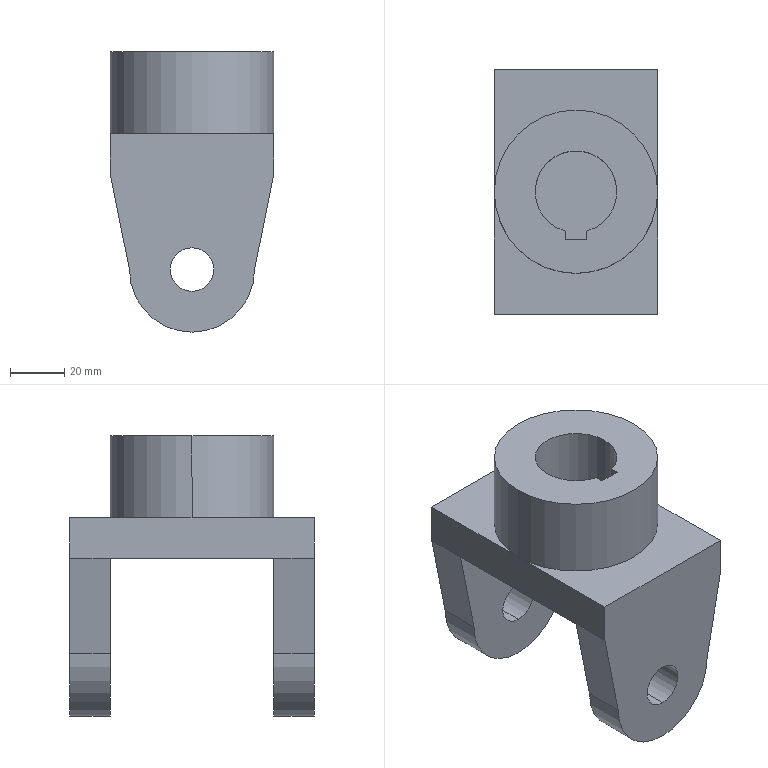Part | SolidWorks | features ICE 2, Extrusion 1, MirrorPattern 1 | 1 solid | 30 faces | box 60 x 90 x 103 mm | volume 218531 mm3 | plane 18 | cylinder 12 | commonest cylinder face diameters 16 x4 30 x3 46 x3 60 x2
STEP:
#1=CARTESIAN_POINT('',(4.,-14.457,30.));
#2=VERTEX_POINT('',#1);
#3=CARTESIAN_POINT('',(15.,0.,30.));
#4=VERTEX_POINT('',#3);
#5=CARTESIAN_POINT('',(0.,0.,30.));
#6=DIRECTION('',(0.,0.,1.));
#7=DIRECTION('',(1.,0.,0.));
#8=AXIS2_PLACEMENT_3D('',#5,#6,#7);
#9=CIRCLE('',#8,15.);
#10=EDGE_CURVE('',#2,#4,#9,.T.);
#11=ORIENTED_EDGE('',*,*,#10,.T.);
#12=CARTESIAN_POINT('',(15.,0.,0.));
#13=VERTEX_POINT('',#12);
#14=CARTESIAN_POINT('',(15.,0.,30.));
#15=DIRECTION('',(0.,0.,-1.));
#16=VECTOR('',#15,1000.);
#17=LINE('',#14,#16);
#18=EDGE_CURVE('',#4,#13,#17,.T.);
#19=ORIENTED_EDGE('',*,*,#18,.T.);
#20=CARTESIAN_POINT('',(4.,-14.457,0.));
#21=VERTEX_POINT('',#20);
#22=CARTESIAN_POINT('',(0.,0.,0.));
#23=DIRECTION('',(0.,0.,1.));
#24=DIRECTION('',(1.,0.,0.));
#25=AXIS2_PLACEMENT_3D('',#22,#23,#24);
#26=CIRCLE('',#25,15.);
#27=EDGE_CURVE('',#21,#13,#26,.T.);
#28=ORIENTED_EDGE('',*,*,#27,.F.);
#29=CARTESIAN_POINT('',(4.,-14.457,30.));
#30=DIRECTION('',(0.,0.,-1.));
#31=VECTOR('',#30,1000.);
#32=LINE('',#29,#31);
#33=EDGE_CURVE('',#2,#21,#32,.T.);
#34=ORIENTED_EDGE('',*,*,#33,.F.);
#35=EDGE_LOOP('',(#11,#19,#28,#34));
#36=FACE_OUTER_BOUND('',#35,.T.);
#37=CARTESIAN_POINT('',(0.,0.,30.));
#38=DIRECTION('',(0.,0.,-1.));
#39=DIRECTION('',(-1.,0.,0.));
#40=AXIS2_PLACEMENT_3D('',#37,#38,#39);
#41=CYLINDRICAL_SURFACE('',#40,15.);
#42=ADVANCED_FACE('',(#36),#41,.F.);
#43=ORIENTED_EDGE('',*,*,#18,.F.);
#44=CARTESIAN_POINT('',(-15.,0.,30.));
#45=VERTEX_POINT('',#44);
#46=CARTESIAN_POINT('',(0.,0.,30.));
#47=DIRECTION('',(0.,0.,1.));
#48=DIRECTION('',(1.,0.,0.));
#49=AXIS2_PLACEMENT_3D('',#46,#47,#48);
#50=CIRCLE('',#49,15.);
#51=EDGE_CURVE('',#4,#45,#50,.T.);
#52=ORIENTED_EDGE('',*,*,#51,.T.);
#53=CARTESIAN_POINT('',(-15.,0.,0.));
#54=VERTEX_POINT('',#53);
#55=CARTESIAN_POINT('',(-15.,0.,30.));
#56=DIRECTION('',(0.,0.,-1.));
#57=VECTOR('',#56,1000.);
#58=LINE('',#55,#57);
#59=EDGE_CURVE('',#45,#54,#58,.T.);
#60=ORIENTED_EDGE('',*,*,#59,.T.);
#61=CARTESIAN_POINT('',(0.,0.,0.));
#62=DIRECTION('',(0.,0.,1.));
#63=DIRECTION('',(1.,0.,0.));
#64=AXIS2_PLACEMENT_3D('',#61,#62,#63);
#65=CIRCLE('',#64,15.);
#66=EDGE_CURVE('',#13,#54,#65,.T.);
#67=ORIENTED_EDGE('',*,*,#66,.F.);
#68=EDGE_LOOP('',(#43,#52,#60,#67));
#69=FACE_OUTER_BOUND('',#68,.T.);
#70=CARTESIAN_POINT('',(0.,0.,30.));
#71=DIRECTION('',(0.,0.,-1.));
#72=DIRECTION('',(-1.,0.,0.));
#73=AXIS2_PLACEMENT_3D('',#70,#71,#72);
#74=CYLINDRICAL_SURFACE('',#73,15.);
#75=ADVANCED_FACE('',(#69),#74,.F.);
#76=CARTESIAN_POINT('',(30.,0.,30.));
#77=VERTEX_POINT('',#76);
#78=CARTESIAN_POINT('',(-30.,0.,30.));
#79=VERTEX_POINT('',#78);
#80=CARTESIAN_POINT('',(0.,0.,30.));
#81=DIRECTION('',(0.,0.,1.));
#82=DIRECTION('',(1.,0.,0.));
#83=AXIS2_PLACEMENT_3D('',#80,#81,#82);
#84=CIRCLE('',#83,30.);
#85=EDGE_CURVE('',#77,#79,#84,.T.);
#86=ORIENTED_EDGE('',*,*,#85,.F.);
#87=CARTESIAN_POINT('',(30.,0.,0.));
#88=VERTEX_POINT('',#87);
#89=CARTESIAN_POINT('',(30.,0.,30.));
#90=DIRECTION('',(0.,0.,-1.));
#91=VECTOR('',#90,1000.);
#92=LINE('',#89,#91);
#93=EDGE_CURVE('',#77,#88,#92,.T.);
#94=ORIENTED_EDGE('',*,*,#93,.T.);
#95=CARTESIAN_POINT('',(-30.,0.,0.));
#96=VERTEX_POINT('',#95);
#97=CARTESIAN_POINT('',(0.,0.,0.));
#98=DIRECTION('',(0.,0.,1.));
#99=DIRECTION('',(1.,0.,0.));
#100=AXIS2_PLACEMENT_3D('',#97,#98,#99);
#101=CIRCLE('',#100,30.);
#102=EDGE_CURVE('',#88,#96,#101,.T.);
#103=ORIENTED_EDGE('',*,*,#102,.T.);
#104=CARTESIAN_POINT('',(-30.,0.,30.));
#105=DIRECTION('',(0.,0.,-1.));
#106=VECTOR('',#105,1000.);
#107=LINE('',#104,#106);
#108=EDGE_CURVE('',#79,#96,#107,.T.);
#109=ORIENTED_EDGE('',*,*,#108,.F.);
#110=EDGE_LOOP('',(#86,#94,#103,#109));
#111=FACE_OUTER_BOUND('',#110,.T.);
#112=CARTESIAN_POINT('',(0.,0.,30.));
#113=DIRECTION('',(0.,0.,-1.));
#114=DIRECTION('',(-1.,0.,0.));
#115=AXIS2_PLACEMENT_3D('',#112,#113,#114);
#116=CYLINDRICAL_SURFACE('',#115,30.);
#117=ADVANCED_FACE('',(#111),#116,.T.);
#118=CARTESIAN_POINT('',(0.,-30.,-58.));
#119=VERTEX_POINT('',#118);
#120=CARTESIAN_POINT('',(0.,-30.,-42.));
#121=VERTEX_POINT('',#120);
#122=CARTESIAN_POINT('',(0.,-30.,-50.));
#123=DIRECTION('',(0.,1.,0.));
#124=DIRECTION('',(0.,0.,1.));
#125=AXIS2_PLACEMENT_3D('',#122,#123,#124);
#126=CIRCLE('',#125,8.);
#127=EDGE_CURVE('',#119,#121,#126,.T.);
#128=ORIENTED_EDGE('',*,*,#127,.T.);
#129=CARTESIAN_POINT('',(0.,-45.,-42.));
#130=VERTEX_POINT('',#129);
#131=CARTESIAN_POINT('',(0.,-30.,-42.));
#132=DIRECTION('',(0.,-1.,0.));
#133=VECTOR('',#132,1000.);
#134=LINE('',#131,#133);
#135=EDGE_CURVE('',#121,#130,#134,.T.);
#136=ORIENTED_EDGE('',*,*,#135,.T.);
#137=CARTESIAN_POINT('',(0.,-45.,-58.));
#138=VERTEX_POINT('',#137);
#139=CARTESIAN_POINT('',(0.,-45.,-50.));
#140=DIRECTION('',(0.,1.,0.));
#141=DIRECTION('',(0.,0.,1.));
#142=AXIS2_PLACEMENT_3D('',#139,#140,#141);
#143=CIRCLE('',#142,8.);
#144=EDGE_CURVE('',#138,#130,#143,.T.);
#145=ORIENTED_EDGE('',*,*,#144,.F.);
#146=CARTESIAN_POINT('',(0.,-30.,-58.));
#147=DIRECTION('',(0.,-1.,0.));
#148=VECTOR('',#147,1000.);
#149=LINE('',#146,#148);
#150=EDGE_CURVE('',#119,#138,#149,.T.);
#151=ORIENTED_EDGE('',*,*,#150,.F.);
#152=EDGE_LOOP('',(#128,#136,#145,#151));
#153=FACE_OUTER_BOUND('',#152,.T.);
#154=CARTESIAN_POINT('',(0.,-30.,-50.));
#155=DIRECTION('',(0.,-1.,0.));
#156=DIRECTION('',(0.,0.,-1.));
#157=AXIS2_PLACEMENT_3D('',#154,#155,#156);
#158=CYLINDRICAL_SURFACE('',#157,8.);
#159=ADVANCED_FACE('',(#153),#158,.F.);
#160=CARTESIAN_POINT('',(0.,-30.,-73.));
#161=VERTEX_POINT('',#160);
#162=CARTESIAN_POINT('',(-23.,-30.,-50.));
#163=VERTEX_POINT('',#162);
#164=CARTESIAN_POINT('',(0.,-30.,-50.));
#165=DIRECTION('',(0.,1.,0.));
#166=DIRECTION('',(0.,0.,1.));
#167=AXIS2_PLACEMENT_3D('',#164,#165,#166);
#168=CIRCLE('',#167,23.);
#169=EDGE_CURVE('',#161,#163,#168,.T.);
#170=ORIENTED_EDGE('',*,*,#169,.F.);
#171=CARTESIAN_POINT('',(0.,-45.,-73.));
#172=VERTEX_POINT('',#171);
#173=CARTESIAN_POINT('',(0.,-30.,-73.));
#174=DIRECTION('',(0.,-1.,0.));
#175=VECTOR('',#174,1000.);
#176=LINE('',#173,#175);
#177=EDGE_CURVE('',#161,#172,#176,.T.);
#178=ORIENTED_EDGE('',*,*,#177,.T.);
#179=CARTESIAN_POINT('',(-23.,-45.,-50.));
#180=VERTEX_POINT('',#179);
#181=CARTESIAN_POINT('',(0.,-45.,-50.));
#182=DIRECTION('',(0.,1.,0.));
#183=DIRECTION('',(0.,0.,1.));
#184=AXIS2_PLACEMENT_3D('',#181,#182,#183);
#185=CIRCLE('',#184,23.);
#186=EDGE_CURVE('',#172,#180,#185,.T.);
#187=ORIENTED_EDGE('',*,*,#186,.T.);
#188=CARTESIAN_POINT('',(-23.,-30.,-50.));
#189=DIRECTION('',(0.,-1.,0.));
#190=VECTOR('',#189,1000.);
#191=LINE('',#188,#190);
#192=EDGE_CURVE('',#163,#180,#191,.T.);
#193=ORIENTED_EDGE('',*,*,#192,.F.);
#194=EDGE_LOOP('',(#170,#178,#187,#193));
#195=FACE_OUTER_BOUND('',#194,.T.);
#196=CARTESIAN_POINT('',(0.,-30.,-50.));
#197=DIRECTION('',(0.,-1.,0.));
#198=DIRECTION('',(0.,0.,-1.));
#199=AXIS2_PLACEMENT_3D('',#196,#197,#198);
#200=CYLINDRICAL_SURFACE('',#199,23.);
#201=ADVANCED_FACE('',(#195),#200,.T.);
#202=CARTESIAN_POINT('',(0.,30.,-58.));
#203=VERTEX_POINT('',#202);
#204=CARTESIAN_POINT('',(0.,30.,-42.));
#205=VERTEX_POINT('',#204);
#206=CARTESIAN_POINT('',(0.,30.,-50.));
#207=DIRECTION('',(0.,1.,0.));
#208=DIRECTION('',(0.,0.,1.));
#209=AXIS2_PLACEMENT_3D('',#206,#207,#208);
#210=CIRCLE('',#209,8.);
#211=EDGE_CURVE('',#203,#205,#210,.T.);
#212=ORIENTED_EDGE('',*,*,#211,.F.);
#213=CARTESIAN_POINT('',(0.,45.,-58.));
#214=VERTEX_POINT('',#213);
#215=CARTESIAN_POINT('',(0.,30.,-58.));
#216=DIRECTION('',(0.,1.,0.));
#217=VECTOR('',#216,1000.);
#218=LINE('',#215,#217);
#219=EDGE_CURVE('',#203,#214,#218,.T.);
#220=ORIENTED_EDGE('',*,*,#219,.T.);
#221=CARTESIAN_POINT('',(0.,45.,-42.));
#222=VERTEX_POINT('',#221);
#223=CARTESIAN_POINT('',(0.,45.,-50.));
#224=DIRECTION('',(0.,1.,0.));
#225=DIRECTION('',(0.,0.,1.));
#226=AXIS2_PLACEMENT_3D('',#223,#224,#225);
#227=CIRCLE('',#226,8.);
#228=EDGE_CURVE('',#214,#222,#227,.T.);
#229=ORIENTED_EDGE('',*,*,#228,.T.);
#230=CARTESIAN_POINT('',(0.,30.,-42.));
#231=DIRECTION('',(0.,1.,0.));
#232=VECTOR('',#231,1000.);
#233=LINE('',#230,#232);
#234=EDGE_CURVE('',#205,#222,#233,.T.);
#235=ORIENTED_EDGE('',*,*,#234,.F.);
#236=EDGE_LOOP('',(#212,#220,#229,#235));
#237=FACE_OUTER_BOUND('',#236,.T.);
#238=CARTESIAN_POINT('',(0.,30.,-50.));
#239=DIRECTION('',(0.,1.,0.));
#240=DIRECTION('',(0.,0.,1.));
#241=AXIS2_PLACEMENT_3D('',#238,#239,#240);
#242=CYLINDRICAL_SURFACE('',#241,8.);
#243=ADVANCED_FACE('',(#237),#242,.F.);
#244=ORIENTED_EDGE('',*,*,#102,.F.);
#245=CARTESIAN_POINT('',(30.,45.,0.));
#246=VERTEX_POINT('',#245);
#247=CARTESIAN_POINT('',(30.,45.,0.));
#248=DIRECTION('',(0.,1.,0.));
#249=VECTOR('',#248,1000.);
#250=LINE('',#247,#249);
#251=EDGE_CURVE('',#88,#246,#250,.T.);
#252=ORIENTED_EDGE('',*,*,#251,.T.);
#253=CARTESIAN_POINT('',(-30.,45.,0.));
#254=VERTEX_POINT('',#253);
#255=CARTESIAN_POINT('',(-30.,45.,0.));
#256=DIRECTION('',(-1.,0.,0.));
#257=VECTOR('',#256,1000.);
#258=LINE('',#255,#257);
#259=EDGE_CURVE('',#246,#254,#258,.T.);
#260=ORIENTED_EDGE('',*,*,#259,.T.);
#261=CARTESIAN_POINT('',(-30.,45.,0.));
#262=DIRECTION('',(0.,-1.,0.));
#263=VECTOR('',#262,1000.);
#264=LINE('',#261,#263);
#265=EDGE_CURVE('',#254,#96,#264,.T.);
#266=ORIENTED_EDGE('',*,*,#265,.T.);
#267=EDGE_LOOP('',(#244,#252,#260,#266));
#268=FACE_OUTER_BOUND('',#267,.T.);
#269=CARTESIAN_POINT('',(0.,0.,0.));
#270=DIRECTION('',(0.,0.,1.));
#271=DIRECTION('',(1.,0.,0.));
#272=AXIS2_PLACEMENT_3D('',#269,#270,#271);
#273=PLANE('',#272);
#274=ADVANCED_FACE('',(#268),#273,.T.);
#275=CARTESIAN_POINT('',(-30.,-30.,-15.));
#276=VERTEX_POINT('',#275);
#277=CARTESIAN_POINT('',(30.,-30.,-15.));
#278=VERTEX_POINT('',#277);
#279=CARTESIAN_POINT('',(-30.,-30.,-15.));
#280=DIRECTION('',(1.,0.,0.));
#281=VECTOR('',#280,1000.);
#282=LINE('',#279,#281);
#283=EDGE_CURVE('',#276,#278,#282,.T.);
#284=ORIENTED_EDGE('',*,*,#283,.F.);
#285=CARTESIAN_POINT('',(-30.,30.,-15.));
#286=VERTEX_POINT('',#285);
#287=CARTESIAN_POINT('',(-30.,45.,-15.));
#288=DIRECTION('',(0.,-1.,0.));
#289=VECTOR('',#288,1000.);
#290=LINE('',#287,#289);
#291=EDGE_CURVE('',#286,#276,#290,.T.);
#292=ORIENTED_EDGE('',*,*,#291,.F.);
#293=CARTESIAN_POINT('',(30.,30.,-15.));
#294=VERTEX_POINT('',#293);
#295=CARTESIAN_POINT('',(-30.,30.,-15.));
#296=DIRECTION('',(1.,0.,0.));
#297=VECTOR('',#296,1000.);
#298=LINE('',#295,#297);
#299=EDGE_CURVE('',#286,#294,#298,.T.);
#300=ORIENTED_EDGE('',*,*,#299,.T.);
#301=CARTESIAN_POINT('',(30.,45.,-15.));
#302=DIRECTION('',(0.,1.,0.));
#303=VECTOR('',#302,1000.);
#304=LINE('',#301,#303);
#305=EDGE_CURVE('',#278,#294,#304,.T.);
#306=ORIENTED_EDGE('',*,*,#305,.F.);
#307=EDGE_LOOP('',(#284,#292,#300,#306));
#308=FACE_OUTER_BOUND('',#307,.T.);
#309=CARTESIAN_POINT('',(0.,0.,-15.));
#310=DIRECTION('',(0.,0.,1.));
#311=DIRECTION('',(1.,0.,0.));
#312=AXIS2_PLACEMENT_3D('',#309,#310,#311);
#313=PLANE('',#312);
#314=ADVANCED_FACE('',(#308),#313,.F.);
#315=CARTESIAN_POINT('',(30.,-45.,0.));
#316=VERTEX_POINT('',#315);
#317=CARTESIAN_POINT('',(30.,45.,0.));
#318=DIRECTION('',(0.,1.,0.));
#319=VECTOR('',#318,1000.);
#320=LINE('',#317,#319);
#321=EDGE_CURVE('',#316,#88,#320,.T.);
#322=ORIENTED_EDGE('',*,*,#321,.F.);
#323=CARTESIAN_POINT('',(30.,-45.,-15.));
#324=VERTEX_POINT('',#323);
#325=CARTESIAN_POINT('',(30.,-45.,-15.));
#326=DIRECTION('',(0.,0.,1.));
#327=VECTOR('',#326,1000.);
#328=LINE('',#325,#327);
#329=EDGE_CURVE('',#324,#316,#328,.T.);
#330=ORIENTED_EDGE('',*,*,#329,.F.);
#331=CARTESIAN_POINT('',(30.,45.,-15.));
#332=DIRECTION('',(0.,1.,0.));
#333=VECTOR('',#332,1000.);
#334=LINE('',#331,#333);
#335=EDGE_CURVE('',#324,#278,#334,.T.);
#336=ORIENTED_EDGE('',*,*,#335,.T.);
#337=ORIENTED_EDGE('',*,*,#305,.T.);
#338=CARTESIAN_POINT('',(30.,45.,-15.));
#339=VERTEX_POINT('',#338);
#340=CARTESIAN_POINT('',(30.,30.,-15.));
#341=DIRECTION('',(0.,1.,0.));
#342=VECTOR('',#341,1000.);
#343=LINE('',#340,#342);
#344=EDGE_CURVE('',#294,#339,#343,.T.);
#345=ORIENTED_EDGE('',*,*,#344,.T.);
#346=CARTESIAN_POINT('',(30.,45.,-15.));
#347=DIRECTION('',(0.,0.,1.));
#348=VECTOR('',#347,1000.);
#349=LINE('',#346,#348);
#350=EDGE_CURVE('',#339,#246,#349,.T.);
#351=ORIENTED_EDGE('',*,*,#350,.T.);
#352=ORIENTED_EDGE('',*,*,#251,.F.);
#353=EDGE_LOOP('',(#322,#330,#336,#337,#345,#351,#352));
#354=FACE_OUTER_BOUND('',#353,.T.);
#355=CARTESIAN_POINT('',(30.,45.,-15.));
#356=DIRECTION('',(1.,0.,0.));
#357=DIRECTION('',(0.,1.,0.));
#358=AXIS2_PLACEMENT_3D('',#355,#356,#357);
#359=PLANE('',#358);
#360=ADVANCED_FACE('',(#354),#359,.T.);
#361=CARTESIAN_POINT('',(-30.,-45.,0.));
#362=VERTEX_POINT('',#361);
#363=CARTESIAN_POINT('',(-30.,-45.,0.));
#364=DIRECTION('',(1.,0.,0.));
#365=VECTOR('',#364,1000.);
#366=LINE('',#363,#365);
#367=EDGE_CURVE('',#362,#316,#366,.T.);
#368=ORIENTED_EDGE('',*,*,#367,.F.);
#369=CARTESIAN_POINT('',(-30.,-45.,-15.));
#370=VERTEX_POINT('',#369);
#371=CARTESIAN_POINT('',(-30.,-45.,-15.));
#372=DIRECTION('',(0.,0.,1.));
#373=VECTOR('',#372,1000.);
#374=LINE('',#371,#373);
#375=EDGE_CURVE('',#370,#362,#374,.T.);
#376=ORIENTED_EDGE('',*,*,#375,.F.);
#377=CARTESIAN_POINT('',(-23.,-45.,-50.));
#378=DIRECTION('',(-0.1961,0.,0.9806));
#379=VECTOR('',#378,1000.);
#380=LINE('',#377,#379);
#381=EDGE_CURVE('',#180,#370,#380,.T.);
#382=ORIENTED_EDGE('',*,*,#381,.F.);
#383=ORIENTED_EDGE('',*,*,#186,.F.);
#384=CARTESIAN_POINT('',(23.,-45.,-50.));
#385=VERTEX_POINT('',#384);
#386=CARTESIAN_POINT('',(0.,-45.,-50.));
#387=DIRECTION('',(0.,1.,0.));
#388=DIRECTION('',(0.,0.,1.));
#389=AXIS2_PLACEMENT_3D('',#386,#387,#388);
#390=CIRCLE('',#389,23.);
#391=EDGE_CURVE('',#385,#172,#390,.T.);
#392=ORIENTED_EDGE('',*,*,#391,.F.);
#393=CARTESIAN_POINT('',(30.,-45.,-15.));
#394=DIRECTION('',(-0.1961,0.,-0.9806));
#395=VECTOR('',#394,1000.);
#396=LINE('',#393,#395);
#397=EDGE_CURVE('',#324,#385,#396,.T.);
#398=ORIENTED_EDGE('',*,*,#397,.F.);
#399=ORIENTED_EDGE('',*,*,#329,.T.);
#400=EDGE_LOOP('',(#368,#376,#382,#383,#392,#398,#399));
#401=FACE_OUTER_BOUND('',#400,.T.);
#402=ORIENTED_EDGE('',*,*,#144,.T.);
#403=CARTESIAN_POINT('',(0.,-45.,-50.));
#404=DIRECTION('',(0.,1.,0.));
#405=DIRECTION('',(0.,0.,1.));
#406=AXIS2_PLACEMENT_3D('',#403,#404,#405);
#407=CIRCLE('',#406,8.);
#408=EDGE_CURVE('',#130,#138,#407,.T.);
#409=ORIENTED_EDGE('',*,*,#408,.T.);
#410=EDGE_LOOP('',(#402,#409));
#411=FACE_BOUND('',#410,.T.);
#412=CARTESIAN_POINT('',(-30.,-45.,-15.));
#413=DIRECTION('',(0.,-1.,0.));
#414=DIRECTION('',(0.,0.,-1.));
#415=AXIS2_PLACEMENT_3D('',#412,#413,#414);
#416=PLANE('',#415);
#417=ADVANCED_FACE('',(#401,#411),#416,.T.);
#418=ORIENTED_EDGE('',*,*,#265,.F.);
#419=CARTESIAN_POINT('',(-30.,45.,-15.));
#420=VERTEX_POINT('',#419);
#421=CARTESIAN_POINT('',(-30.,45.,-15.));
#422=DIRECTION('',(0.,0.,1.));
#423=VECTOR('',#422,1000.);
#424=LINE('',#421,#423);
#425=EDGE_CURVE('',#420,#254,#424,.T.);
#426=ORIENTED_EDGE('',*,*,#425,.F.);
#427=CARTESIAN_POINT('',(-30.,45.,-15.));
#428=DIRECTION('',(0.,-1.,0.));
#429=VECTOR('',#428,1000.);
#430=LINE('',#427,#429);
#431=EDGE_CURVE('',#420,#286,#430,.T.);
#432=ORIENTED_EDGE('',*,*,#431,.T.);
#433=ORIENTED_EDGE('',*,*,#291,.T.);
#434=CARTESIAN_POINT('',(-30.,-30.,-15.));
#435=DIRECTION('',(0.,-1.,0.));
#436=VECTOR('',#435,1000.);
#437=LINE('',#434,#436);
#438=EDGE_CURVE('',#276,#370,#437,.T.);
#439=ORIENTED_EDGE('',*,*,#438,.T.);
#440=ORIENTED_EDGE('',*,*,#375,.T.);
#441=CARTESIAN_POINT('',(-30.,45.,0.));
#442=DIRECTION('',(0.,-1.,0.));
#443=VECTOR('',#442,1000.);
#444=LINE('',#441,#443);
#445=EDGE_CURVE('',#96,#362,#444,.T.);
#446=ORIENTED_EDGE('',*,*,#445,.F.);
#447=EDGE_LOOP('',(#418,#426,#432,#433,#439,#440,#446));
#448=FACE_OUTER_BOUND('',#447,.T.);
#449=CARTESIAN_POINT('',(-30.,45.,-15.));
#450=DIRECTION('',(-1.,0.,0.));
#451=DIRECTION('',(0.,-1.,0.));
#452=AXIS2_PLACEMENT_3D('',#449,#450,#451);
#453=PLANE('',#452);
#454=ADVANCED_FACE('',(#448),#453,.T.);
#455=ORIENTED_EDGE('',*,*,#259,.F.);
#456=ORIENTED_EDGE('',*,*,#350,.F.);
#457=CARTESIAN_POINT('',(23.,45.,-50.));
#458=VERTEX_POINT('',#457);
#459=CARTESIAN_POINT('',(30.,45.,-15.));
#460=DIRECTION('',(-0.1961,0.,-0.9806));
#461=VECTOR('',#460,1000.);
#462=LINE('',#459,#461);
#463=EDGE_CURVE('',#339,#458,#462,.T.);
#464=ORIENTED_EDGE('',*,*,#463,.T.);
#465=CARTESIAN_POINT('',(-23.,45.,-50.));
#466=VERTEX_POINT('',#465);
#467=CARTESIAN_POINT('',(0.,45.,-50.));
#468=DIRECTION('',(0.,1.,0.));
#469=DIRECTION('',(0.,0.,1.));
#470=AXIS2_PLACEMENT_3D('',#467,#468,#469);
#471=CIRCLE('',#470,23.);
#472=EDGE_CURVE('',#458,#466,#471,.T.);
#473=ORIENTED_EDGE('',*,*,#472,.T.);
#474=CARTESIAN_POINT('',(-23.,45.,-50.));
#475=DIRECTION('',(-0.1961,0.,0.9806));
#476=VECTOR('',#475,1000.);
#477=LINE('',#474,#476);
#478=EDGE_CURVE('',#466,#420,#477,.T.);
#479=ORIENTED_EDGE('',*,*,#478,.T.);
#480=ORIENTED_EDGE('',*,*,#425,.T.);
#481=EDGE_LOOP('',(#455,#456,#464,#473,#479,#480));
#482=FACE_OUTER_BOUND('',#481,.T.);
#483=CARTESIAN_POINT('',(0.,45.,-50.));
#484=DIRECTION('',(0.,1.,0.));
#485=DIRECTION('',(0.,0.,1.));
#486=AXIS2_PLACEMENT_3D('',#483,#484,#485);
#487=CIRCLE('',#486,8.);
#488=EDGE_CURVE('',#222,#214,#487,.T.);
#489=ORIENTED_EDGE('',*,*,#488,.F.);
#490=ORIENTED_EDGE('',*,*,#228,.F.);
#491=EDGE_LOOP('',(#489,#490));
#492=FACE_BOUND('',#491,.T.);
#493=CARTESIAN_POINT('',(-30.,45.,-15.));
#494=DIRECTION('',(0.,1.,0.));
#495=DIRECTION('',(0.,0.,1.));
#496=AXIS2_PLACEMENT_3D('',#493,#494,#495);
#497=PLANE('',#496);
#498=ADVANCED_FACE('',(#482,#492),#497,.T.);
#499=CARTESIAN_POINT('',(0.,0.,0.));
#500=DIRECTION('',(0.,0.,1.));
#501=DIRECTION('',(1.,0.,0.));
#502=AXIS2_PLACEMENT_3D('',#499,#500,#501);
#503=CIRCLE('',#502,30.);
#504=EDGE_CURVE('',#96,#88,#503,.T.);
#505=ORIENTED_EDGE('',*,*,#504,.F.);
#506=ORIENTED_EDGE('',*,*,#445,.T.);
#507=ORIENTED_EDGE('',*,*,#367,.T.);
#508=ORIENTED_EDGE('',*,*,#321,.T.);
#509=EDGE_LOOP('',(#505,#506,#507,#508));
#510=FACE_OUTER_BOUND('',#509,.T.);
#511=CARTESIAN_POINT('',(0.,0.,0.));
#512=DIRECTION('',(0.,0.,1.));
#513=DIRECTION('',(1.,0.,0.));
#514=AXIS2_PLACEMENT_3D('',#511,#512,#513);
#515=PLANE('',#514);
#516=ADVANCED_FACE('',(#510),#515,.T.);
#517=ORIENTED_EDGE('',*,*,#478,.F.);
#518=CARTESIAN_POINT('',(-23.,30.,-50.));
#519=VERTEX_POINT('',#518);
#520=CARTESIAN_POINT('',(-23.,30.,-50.));
#521=DIRECTION('',(0.,1.,0.));
#522=VECTOR('',#521,1000.);
#523=LINE('',#520,#522);
#524=EDGE_CURVE('',#519,#466,#523,.T.);
#525=ORIENTED_EDGE('',*,*,#524,.F.);
#526=CARTESIAN_POINT('',(-23.,30.,-50.));
#527=DIRECTION('',(-0.1961,0.,0.9806));
#528=VECTOR('',#527,1000.);
#529=LINE('',#526,#528);
#530=EDGE_CURVE('',#519,#286,#529,.T.);
#531=ORIENTED_EDGE('',*,*,#530,.T.);
#532=ORIENTED_EDGE('',*,*,#431,.F.);
#533=EDGE_LOOP('',(#517,#525,#531,#532));
#534=FACE_OUTER_BOUND('',#533,.T.);
#535=CARTESIAN_POINT('',(-23.,30.,-50.));
#536=DIRECTION('',(-0.9806,0.,-0.1961));
#537=DIRECTION('',(-0.1961,0.,0.9806));
#538=AXIS2_PLACEMENT_3D('',#535,#536,#537);
#539=PLANE('',#538);
#540=ADVANCED_FACE('',(#534),#539,.T.);
#541=ORIENTED_EDGE('',*,*,#472,.F.);
#542=CARTESIAN_POINT('',(23.,30.,-50.));
#543=VERTEX_POINT('',#542);
#544=CARTESIAN_POINT('',(23.,30.,-50.));
#545=DIRECTION('',(0.,1.,0.));
#546=VECTOR('',#545,1000.);
#547=LINE('',#544,#546);
#548=EDGE_CURVE('',#543,#458,#547,.T.);
#549=ORIENTED_EDGE('',*,*,#548,.F.);
#550=CARTESIAN_POINT('',(0.,30.,-50.));
#551=DIRECTION('',(0.,1.,0.));
#552=DIRECTION('',(0.,0.,1.));
#553=AXIS2_PLACEMENT_3D('',#550,#551,#552);
#554=CIRCLE('',#553,23.);
#555=EDGE_CURVE('',#543,#519,#554,.T.);
#556=ORIENTED_EDGE('',*,*,#555,.T.);
#557=ORIENTED_EDGE('',*,*,#524,.T.);
#558=EDGE_LOOP('',(#541,#549,#556,#557));
#559=FACE_OUTER_BOUND('',#558,.T.);
#560=CARTESIAN_POINT('',(0.,30.,-50.));
#561=DIRECTION('',(0.,1.,0.));
#562=DIRECTION('',(0.,0.,1.));
#563=AXIS2_PLACEMENT_3D('',#560,#561,#562);
#564=CYLINDRICAL_SURFACE('',#563,23.);
#565=ADVANCED_FACE('',(#559),#564,.T.);
#566=ORIENTED_EDGE('',*,*,#463,.F.);
#567=ORIENTED_EDGE('',*,*,#344,.F.);
#568=CARTESIAN_POINT('',(30.,30.,-15.));
#569=DIRECTION('',(-0.1961,0.,-0.9806));
#570=VECTOR('',#569,1000.);
#571=LINE('',#568,#570);
#572=EDGE_CURVE('',#294,#543,#571,.T.);
#573=ORIENTED_EDGE('',*,*,#572,.T.);
#574=ORIENTED_EDGE('',*,*,#548,.T.);
#575=EDGE_LOOP('',(#566,#567,#573,#574));
#576=FACE_OUTER_BOUND('',#575,.T.);
#577=CARTESIAN_POINT('',(30.,30.,-15.));
#578=DIRECTION('',(0.9806,0.,-0.1961));
#579=DIRECTION('',(-0.1961,0.,-0.9806));
#580=AXIS2_PLACEMENT_3D('',#577,#578,#579);
#581=PLANE('',#580);
#582=ADVANCED_FACE('',(#576),#581,.T.);
#583=CARTESIAN_POINT('',(0.,30.,-50.));
#584=DIRECTION('',(0.,1.,0.));
#585=DIRECTION('',(0.,0.,1.));
#586=AXIS2_PLACEMENT_3D('',#583,#584,#585);
#587=CIRCLE('',#586,8.);
#588=EDGE_CURVE('',#205,#203,#587,.T.);
#589=ORIENTED_EDGE('',*,*,#588,.T.);
#590=ORIENTED_EDGE('',*,*,#211,.T.);
#591=EDGE_LOOP('',(#589,#590));
#592=FACE_BOUND('',#591,.T.);
#593=ORIENTED_EDGE('',*,*,#299,.F.);
#594=ORIENTED_EDGE('',*,*,#530,.F.);
#595=ORIENTED_EDGE('',*,*,#555,.F.);
#596=ORIENTED_EDGE('',*,*,#572,.F.);
#597=EDGE_LOOP('',(#593,#594,#595,#596));
#598=FACE_OUTER_BOUND('',#597,.T.);
#599=CARTESIAN_POINT('',(0.,30.,-50.));
#600=DIRECTION('',(0.,1.,0.));
#601=DIRECTION('',(0.,0.,1.));
#602=AXIS2_PLACEMENT_3D('',#599,#600,#601);
#603=PLANE('',#602);
#604=ADVANCED_FACE('',(#592,#598),#603,.F.);
#605=ORIENTED_EDGE('',*,*,#219,.F.);
#606=ORIENTED_EDGE('',*,*,#588,.F.);
#607=ORIENTED_EDGE('',*,*,#234,.T.);
#608=ORIENTED_EDGE('',*,*,#488,.T.);
#609=EDGE_LOOP('',(#605,#606,#607,#608));
#610=FACE_OUTER_BOUND('',#609,.T.);
#611=CARTESIAN_POINT('',(0.,30.,-50.));
#612=DIRECTION('',(0.,1.,0.));
#613=DIRECTION('',(0.,0.,1.));
#614=AXIS2_PLACEMENT_3D('',#611,#612,#613);
#615=CYLINDRICAL_SURFACE('',#614,8.);
#616=ADVANCED_FACE('',(#610),#615,.F.);
#617=ORIENTED_EDGE('',*,*,#283,.T.);
#618=CARTESIAN_POINT('',(23.,-30.,-50.));
#619=VERTEX_POINT('',#618);
#620=CARTESIAN_POINT('',(30.,-30.,-15.));
#621=DIRECTION('',(-0.1961,0.,-0.9806));
#622=VECTOR('',#621,1000.);
#623=LINE('',#620,#622);
#624=EDGE_CURVE('',#278,#619,#623,.T.);
#625=ORIENTED_EDGE('',*,*,#624,.T.);
#626=CARTESIAN_POINT('',(0.,-30.,-50.));
#627=DIRECTION('',(0.,1.,0.));
#628=DIRECTION('',(0.,0.,1.));
#629=AXIS2_PLACEMENT_3D('',#626,#627,#628);
#630=CIRCLE('',#629,23.);
#631=EDGE_CURVE('',#619,#161,#630,.T.);
#632=ORIENTED_EDGE('',*,*,#631,.T.);
#633=ORIENTED_EDGE('',*,*,#169,.T.);
#634=CARTESIAN_POINT('',(-23.,-30.,-50.));
#635=DIRECTION('',(-0.1961,0.,0.9806));
#636=VECTOR('',#635,1000.);
#637=LINE('',#634,#636);
#638=EDGE_CURVE('',#163,#276,#637,.T.);
#639=ORIENTED_EDGE('',*,*,#638,.T.);
#640=EDGE_LOOP('',(#617,#625,#632,#633,#639));
#641=FACE_OUTER_BOUND('',#640,.T.);
#642=ORIENTED_EDGE('',*,*,#127,.F.);
#643=CARTESIAN_POINT('',(0.,-30.,-50.));
#644=DIRECTION('',(0.,1.,0.));
#645=DIRECTION('',(0.,0.,1.));
#646=AXIS2_PLACEMENT_3D('',#643,#644,#645);
#647=CIRCLE('',#646,8.);
#648=EDGE_CURVE('',#121,#119,#647,.T.);
#649=ORIENTED_EDGE('',*,*,#648,.F.);
#650=EDGE_LOOP('',(#642,#649));
#651=FACE_BOUND('',#650,.T.);
#652=CARTESIAN_POINT('',(0.,-30.,-50.));
#653=DIRECTION('',(0.,-1.,0.));
#654=DIRECTION('',(0.,0.,1.));
#655=AXIS2_PLACEMENT_3D('',#652,#653,#654);
#656=PLANE('',#655);
#657=ADVANCED_FACE('',(#641,#651),#656,.F.);
#658=ORIENTED_EDGE('',*,*,#397,.T.);
#659=CARTESIAN_POINT('',(23.,-30.,-50.));
#660=DIRECTION('',(0.,-1.,0.));
#661=VECTOR('',#660,1000.);
#662=LINE('',#659,#661);
#663=EDGE_CURVE('',#619,#385,#662,.T.);
#664=ORIENTED_EDGE('',*,*,#663,.F.);
#665=ORIENTED_EDGE('',*,*,#624,.F.);
#666=ORIENTED_EDGE('',*,*,#335,.F.);
#667=EDGE_LOOP('',(#658,#664,#665,#666));
#668=FACE_OUTER_BOUND('',#667,.T.);
#669=CARTESIAN_POINT('',(30.,-30.,-15.));
#670=DIRECTION('',(-0.9806,0.,0.1961));
#671=DIRECTION('',(0.1961,0.,0.9806));
#672=AXIS2_PLACEMENT_3D('',#669,#670,#671);
#673=PLANE('',#672);
#674=ADVANCED_FACE('',(#668),#673,.F.);
#675=ORIENTED_EDGE('',*,*,#177,.F.);
#676=ORIENTED_EDGE('',*,*,#631,.F.);
#677=ORIENTED_EDGE('',*,*,#663,.T.);
#678=ORIENTED_EDGE('',*,*,#391,.T.);
#679=EDGE_LOOP('',(#675,#676,#677,#678));
#680=FACE_OUTER_BOUND('',#679,.T.);
#681=CARTESIAN_POINT('',(0.,-30.,-50.));
#682=DIRECTION('',(0.,-1.,0.));
#683=DIRECTION('',(0.,0.,-1.));
#684=AXIS2_PLACEMENT_3D('',#681,#682,#683);
#685=CYLINDRICAL_SURFACE('',#684,23.);
#686=ADVANCED_FACE('',(#680),#685,.T.);
#687=ORIENTED_EDGE('',*,*,#381,.T.);
#688=ORIENTED_EDGE('',*,*,#438,.F.);
#689=ORIENTED_EDGE('',*,*,#638,.F.);
#690=ORIENTED_EDGE('',*,*,#192,.T.);
#691=EDGE_LOOP('',(#687,#688,#689,#690));
#692=FACE_OUTER_BOUND('',#691,.T.);
#693=CARTESIAN_POINT('',(-23.,-30.,-50.));
#694=DIRECTION('',(0.9806,0.,0.1961));
#695=DIRECTION('',(0.1961,0.,-0.9806));
#696=AXIS2_PLACEMENT_3D('',#693,#694,#695);
#697=PLANE('',#696);
#698=ADVANCED_FACE('',(#692),#697,.F.);
#699=ORIENTED_EDGE('',*,*,#135,.F.);
#700=ORIENTED_EDGE('',*,*,#648,.T.);
#701=ORIENTED_EDGE('',*,*,#150,.T.);
#702=ORIENTED_EDGE('',*,*,#408,.F.);
#703=EDGE_LOOP('',(#699,#700,#701,#702));
#704=FACE_OUTER_BOUND('',#703,.T.);
#705=CARTESIAN_POINT('',(0.,-30.,-50.));
#706=DIRECTION('',(0.,-1.,0.));
#707=DIRECTION('',(0.,0.,-1.));
#708=AXIS2_PLACEMENT_3D('',#705,#706,#707);
#709=CYLINDRICAL_SURFACE('',#708,8.);
#710=ADVANCED_FACE('',(#704),#709,.F.);
#711=CARTESIAN_POINT('',(0.,0.,30.));
#712=DIRECTION('',(0.,0.,1.));
#713=DIRECTION('',(1.,0.,0.));
#714=AXIS2_PLACEMENT_3D('',#711,#712,#713);
#715=CIRCLE('',#714,30.);
#716=EDGE_CURVE('',#79,#77,#715,.T.);
#717=ORIENTED_EDGE('',*,*,#716,.T.);
#718=ORIENTED_EDGE('',*,*,#85,.T.);
#719=EDGE_LOOP('',(#717,#718));
#720=FACE_OUTER_BOUND('',#719,.T.);
#721=CARTESIAN_POINT('',(-4.,-14.457,30.));
#722=VERTEX_POINT('',#721);
#723=CARTESIAN_POINT('',(-4.,-17.457,30.));
#724=VERTEX_POINT('',#723);
#725=CARTESIAN_POINT('',(-4.,-14.457,30.));
#726=DIRECTION('',(0.,-1.,0.));
#727=VECTOR('',#726,1000.);
#728=LINE('',#725,#727);
#729=EDGE_CURVE('',#722,#724,#728,.T.);
#730=ORIENTED_EDGE('',*,*,#729,.F.);
#731=CARTESIAN_POINT('',(0.,0.,30.));
#732=DIRECTION('',(0.,0.,1.));
#733=DIRECTION('',(1.,0.,0.));
#734=AXIS2_PLACEMENT_3D('',#731,#732,#733);
#735=CIRCLE('',#734,15.);
#736=EDGE_CURVE('',#45,#722,#735,.T.);
#737=ORIENTED_EDGE('',*,*,#736,.F.);
#738=ORIENTED_EDGE('',*,*,#51,.F.);
#739=ORIENTED_EDGE('',*,*,#10,.F.);
#740=CARTESIAN_POINT('',(4.,-17.457,30.));
#741=VERTEX_POINT('',#740);
#742=CARTESIAN_POINT('',(4.,-14.457,30.));
#743=DIRECTION('',(0.,1.,0.));
#744=VECTOR('',#743,1000.);
#745=LINE('',#742,#744);
#746=EDGE_CURVE('',#741,#2,#745,.T.);
#747=ORIENTED_EDGE('',*,*,#746,.F.);
#748=CARTESIAN_POINT('',(-4.,-17.457,30.));
#749=DIRECTION('',(1.,0.,0.));
#750=VECTOR('',#749,1000.);
#751=LINE('',#748,#750);
#752=EDGE_CURVE('',#724,#741,#751,.T.);
#753=ORIENTED_EDGE('',*,*,#752,.F.);
#754=EDGE_LOOP('',(#730,#737,#738,#739,#747,#753));
#755=FACE_BOUND('',#754,.T.);
#756=CARTESIAN_POINT('',(0.,0.,30.));
#757=DIRECTION('',(0.,0.,1.));
#758=DIRECTION('',(1.,0.,0.));
#759=AXIS2_PLACEMENT_3D('',#756,#757,#758);
#760=PLANE('',#759);
#761=ADVANCED_FACE('',(#720,#755),#760,.T.);
#762=ORIENTED_EDGE('',*,*,#93,.F.);
#763=ORIENTED_EDGE('',*,*,#716,.F.);
#764=ORIENTED_EDGE('',*,*,#108,.T.);
#765=ORIENTED_EDGE('',*,*,#504,.T.);
#766=EDGE_LOOP('',(#762,#763,#764,#765));
#767=FACE_OUTER_BOUND('',#766,.T.);
#768=CARTESIAN_POINT('',(0.,0.,30.));
#769=DIRECTION('',(0.,0.,-1.));
#770=DIRECTION('',(-1.,0.,0.));
#771=AXIS2_PLACEMENT_3D('',#768,#769,#770);
#772=CYLINDRICAL_SURFACE('',#771,30.);
#773=ADVANCED_FACE('',(#767),#772,.T.);
#774=ORIENTED_EDGE('',*,*,#59,.F.);
#775=ORIENTED_EDGE('',*,*,#736,.T.);
#776=CARTESIAN_POINT('',(-4.,-14.457,0.));
#777=VERTEX_POINT('',#776);
#778=CARTESIAN_POINT('',(-4.,-14.457,30.));
#779=DIRECTION('',(0.,0.,-1.));
#780=VECTOR('',#779,1000.);
#781=LINE('',#778,#780);
#782=EDGE_CURVE('',#722,#777,#781,.T.);
#783=ORIENTED_EDGE('',*,*,#782,.T.);
#784=CARTESIAN_POINT('',(0.,0.,0.));
#785=DIRECTION('',(0.,0.,1.));
#786=DIRECTION('',(1.,0.,0.));
#787=AXIS2_PLACEMENT_3D('',#784,#785,#786);
#788=CIRCLE('',#787,15.);
#789=EDGE_CURVE('',#54,#777,#788,.T.);
#790=ORIENTED_EDGE('',*,*,#789,.F.);
#791=EDGE_LOOP('',(#774,#775,#783,#790));
#792=FACE_OUTER_BOUND('',#791,.T.);
#793=CARTESIAN_POINT('',(0.,0.,30.));
#794=DIRECTION('',(0.,0.,-1.));
#795=DIRECTION('',(-1.,0.,0.));
#796=AXIS2_PLACEMENT_3D('',#793,#794,#795);
#797=CYLINDRICAL_SURFACE('',#796,15.);
#798=ADVANCED_FACE('',(#792),#797,.F.);
#799=CARTESIAN_POINT('',(-4.,-17.457,0.));
#800=VERTEX_POINT('',#799);
#801=CARTESIAN_POINT('',(-4.,-14.457,0.));
#802=DIRECTION('',(0.,-1.,0.));
#803=VECTOR('',#802,1000.);
#804=LINE('',#801,#803);
#805=EDGE_CURVE('',#777,#800,#804,.T.);
#806=ORIENTED_EDGE('',*,*,#805,.F.);
#807=ORIENTED_EDGE('',*,*,#782,.F.);
#808=ORIENTED_EDGE('',*,*,#729,.T.);
#809=CARTESIAN_POINT('',(-4.,-17.457,30.));
#810=DIRECTION('',(0.,0.,-1.));
#811=VECTOR('',#810,1000.);
#812=LINE('',#809,#811);
#813=EDGE_CURVE('',#724,#800,#812,.T.);
#814=ORIENTED_EDGE('',*,*,#813,.T.);
#815=EDGE_LOOP('',(#806,#807,#808,#814));
#816=FACE_OUTER_BOUND('',#815,.T.);
#817=CARTESIAN_POINT('',(-4.,-14.457,30.));
#818=DIRECTION('',(1.,0.,0.));
#819=DIRECTION('',(0.,0.,-1.));
#820=AXIS2_PLACEMENT_3D('',#817,#818,#819);
#821=PLANE('',#820);
#822=ADVANCED_FACE('',(#816),#821,.T.);
#823=CARTESIAN_POINT('',(4.,-17.457,0.));
#824=VERTEX_POINT('',#823);
#825=CARTESIAN_POINT('',(-4.,-17.457,0.));
#826=DIRECTION('',(1.,0.,0.));
#827=VECTOR('',#826,1000.);
#828=LINE('',#825,#827);
#829=EDGE_CURVE('',#800,#824,#828,.T.);
#830=ORIENTED_EDGE('',*,*,#829,.F.);
#831=ORIENTED_EDGE('',*,*,#813,.F.);
#832=ORIENTED_EDGE('',*,*,#752,.T.);
#833=CARTESIAN_POINT('',(4.,-17.457,30.));
#834=DIRECTION('',(0.,0.,-1.));
#835=VECTOR('',#834,1000.);
#836=LINE('',#833,#835);
#837=EDGE_CURVE('',#741,#824,#836,.T.);
#838=ORIENTED_EDGE('',*,*,#837,.T.);
#839=EDGE_LOOP('',(#830,#831,#832,#838));
#840=FACE_OUTER_BOUND('',#839,.T.);
#841=CARTESIAN_POINT('',(-4.,-17.457,30.));
#842=DIRECTION('',(0.,1.,0.));
#843=DIRECTION('',(0.,0.,1.));
#844=AXIS2_PLACEMENT_3D('',#841,#842,#843);
#845=PLANE('',#844);
#846=ADVANCED_FACE('',(#840),#845,.T.);
#847=CARTESIAN_POINT('',(4.,-14.457,0.));
#848=DIRECTION('',(0.,1.,0.));
#849=VECTOR('',#848,1000.);
#850=LINE('',#847,#849);
#851=EDGE_CURVE('',#824,#21,#850,.T.);
#852=ORIENTED_EDGE('',*,*,#851,.F.);
#853=ORIENTED_EDGE('',*,*,#837,.F.);
#854=ORIENTED_EDGE('',*,*,#746,.T.);
#855=ORIENTED_EDGE('',*,*,#33,.T.);
#856=EDGE_LOOP('',(#852,#853,#854,#855));
#857=FACE_OUTER_BOUND('',#856,.T.);
#858=CARTESIAN_POINT('',(4.,-14.457,30.));
#859=DIRECTION('',(-1.,0.,0.));
#860=DIRECTION('',(0.,-1.,0.));
#861=AXIS2_PLACEMENT_3D('',#858,#859,#860);
#862=PLANE('',#861);
#863=ADVANCED_FACE('',(#857),#862,.T.);
#864=ORIENTED_EDGE('',*,*,#851,.T.);
#865=ORIENTED_EDGE('',*,*,#27,.T.);
#866=ORIENTED_EDGE('',*,*,#66,.T.);
#867=ORIENTED_EDGE('',*,*,#789,.T.);
#868=ORIENTED_EDGE('',*,*,#805,.T.);
#869=ORIENTED_EDGE('',*,*,#829,.T.);
#870=EDGE_LOOP('',(#864,#865,#866,#867,#868,#869));
#871=FACE_OUTER_BOUND('',#870,.T.);
#872=CARTESIAN_POINT('',(0.,0.,0.));
#873=DIRECTION('',(0.,0.,1.));
#874=DIRECTION('',(1.,0.,0.));
#875=AXIS2_PLACEMENT_3D('',#872,#873,#874);
#876=PLANE('',#875);
#877=ADVANCED_FACE('',(#871),#876,.T.);
#878=CLOSED_SHELL('',(#42,#75,#117,#159,#201,#243,#274,#314,#360,#417,#454,#498,#516,#540,#565,#582,#604,#616,#657,#674,#686,#698,#710,#761,#773,#798,#822,#846,#863,#877));
#879=MANIFOLD_SOLID_BREP('',#878);
#880=CARTESIAN_POINT('',(0.,0.,0.));
#881=DIRECTION('',(0.,0.,1.));
#882=DIRECTION('',(1.,0.,0.));
#883=AXIS2_PLACEMENT_3D('',#880,#881,#882);
#884=(LENGTH_UNIT()NAMED_UNIT(*)SI_UNIT(.MILLI.,.METRE.));
#885=UNCERTAINTY_MEASURE_WITH_UNIT(LENGTH_MEASURE(0.00001),#884,'','');
#886=(NAMED_UNIT(*)PLANE_ANGLE_UNIT()SI_UNIT($,.RADIAN.));
#887=(NAMED_UNIT(*)SI_UNIT($,.STERADIAN.)SOLID_ANGLE_UNIT());
#888=(GEOMETRIC_REPRESENTATION_CONTEXT(3)GLOBAL_UNCERTAINTY_ASSIGNED_CONTEXT((#885))GLOBAL_UNIT_ASSIGNED_CONTEXT((#884,#886,#887))REPRESENTATION_CONTEXT('',''));
#889=ADVANCED_BREP_SHAPE_REPRESENTATION('',(#879,#883),#888);